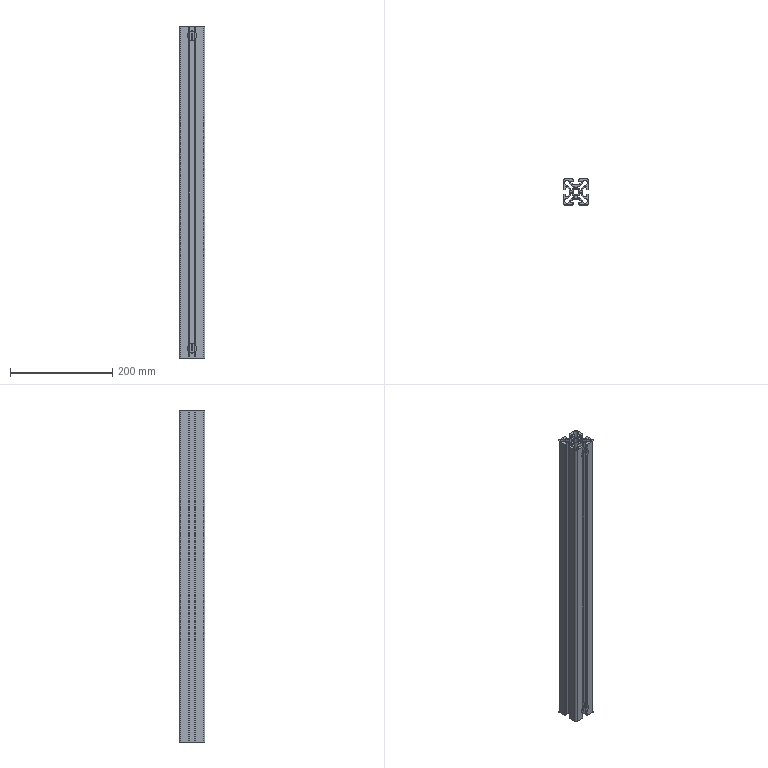Part | NX | features BREP 1 | 1 solid | 231 faces | box 50 x 50 x 650 mm | volume 637784 mm3 | plane 154 | cylinder 77 | commonest cylinder face diameters 2 x37 19 x16 10 x12 6 x4 12 x4 17 x4